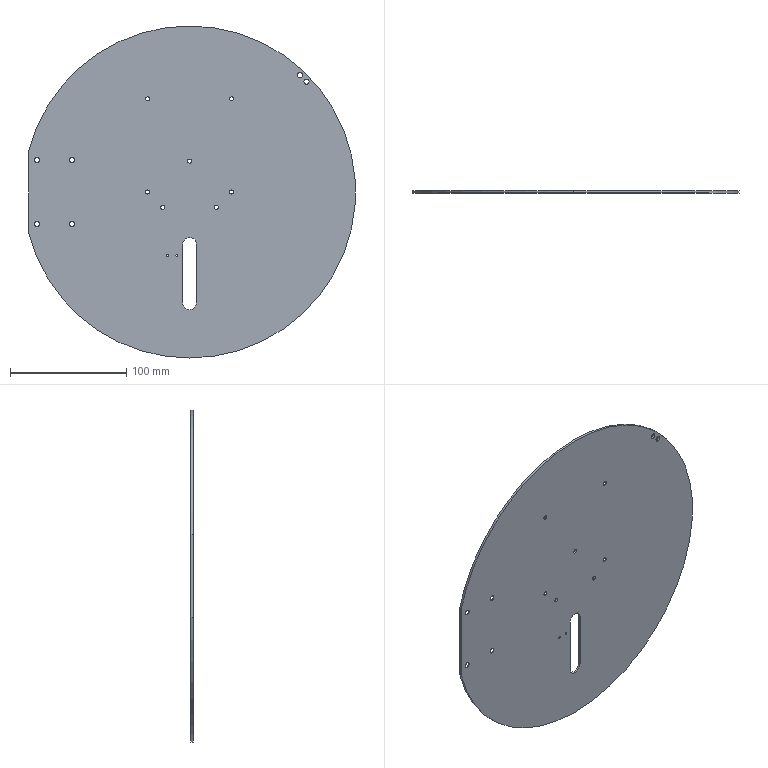Part | SolidWorks | features ICE 3, Chamfer 2, Cut 2, 3DProfileFeature 1, CirPattern 1, Extrusion 1, HoleWzd 1 | 1 solid | 57 faces | box 280.5 x 2 x 285 mm | volume 125189 mm3 | cylinder 36 | cone 16 | plane 5 | commonest cylinder face diameters 3.5 x14 4.5 x12 1.6 x4 12 x3 285 x3